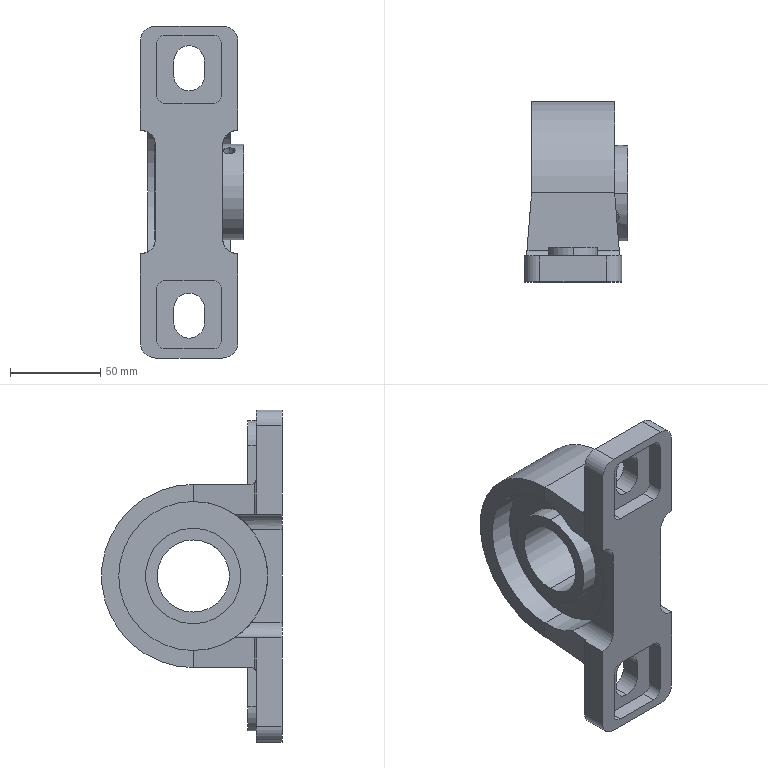Part | STEP file | 果蔬烘干机-208 轴承座 | 1 solid | 91 faces | box 57.2 x 100 x 184 mm | volume 317454 mm3 | cylinder 48 | plane 43 | commonest cylinder face diameters 17 x14 10 x8 2 x4 6 x4 6.647 x4 53 x4